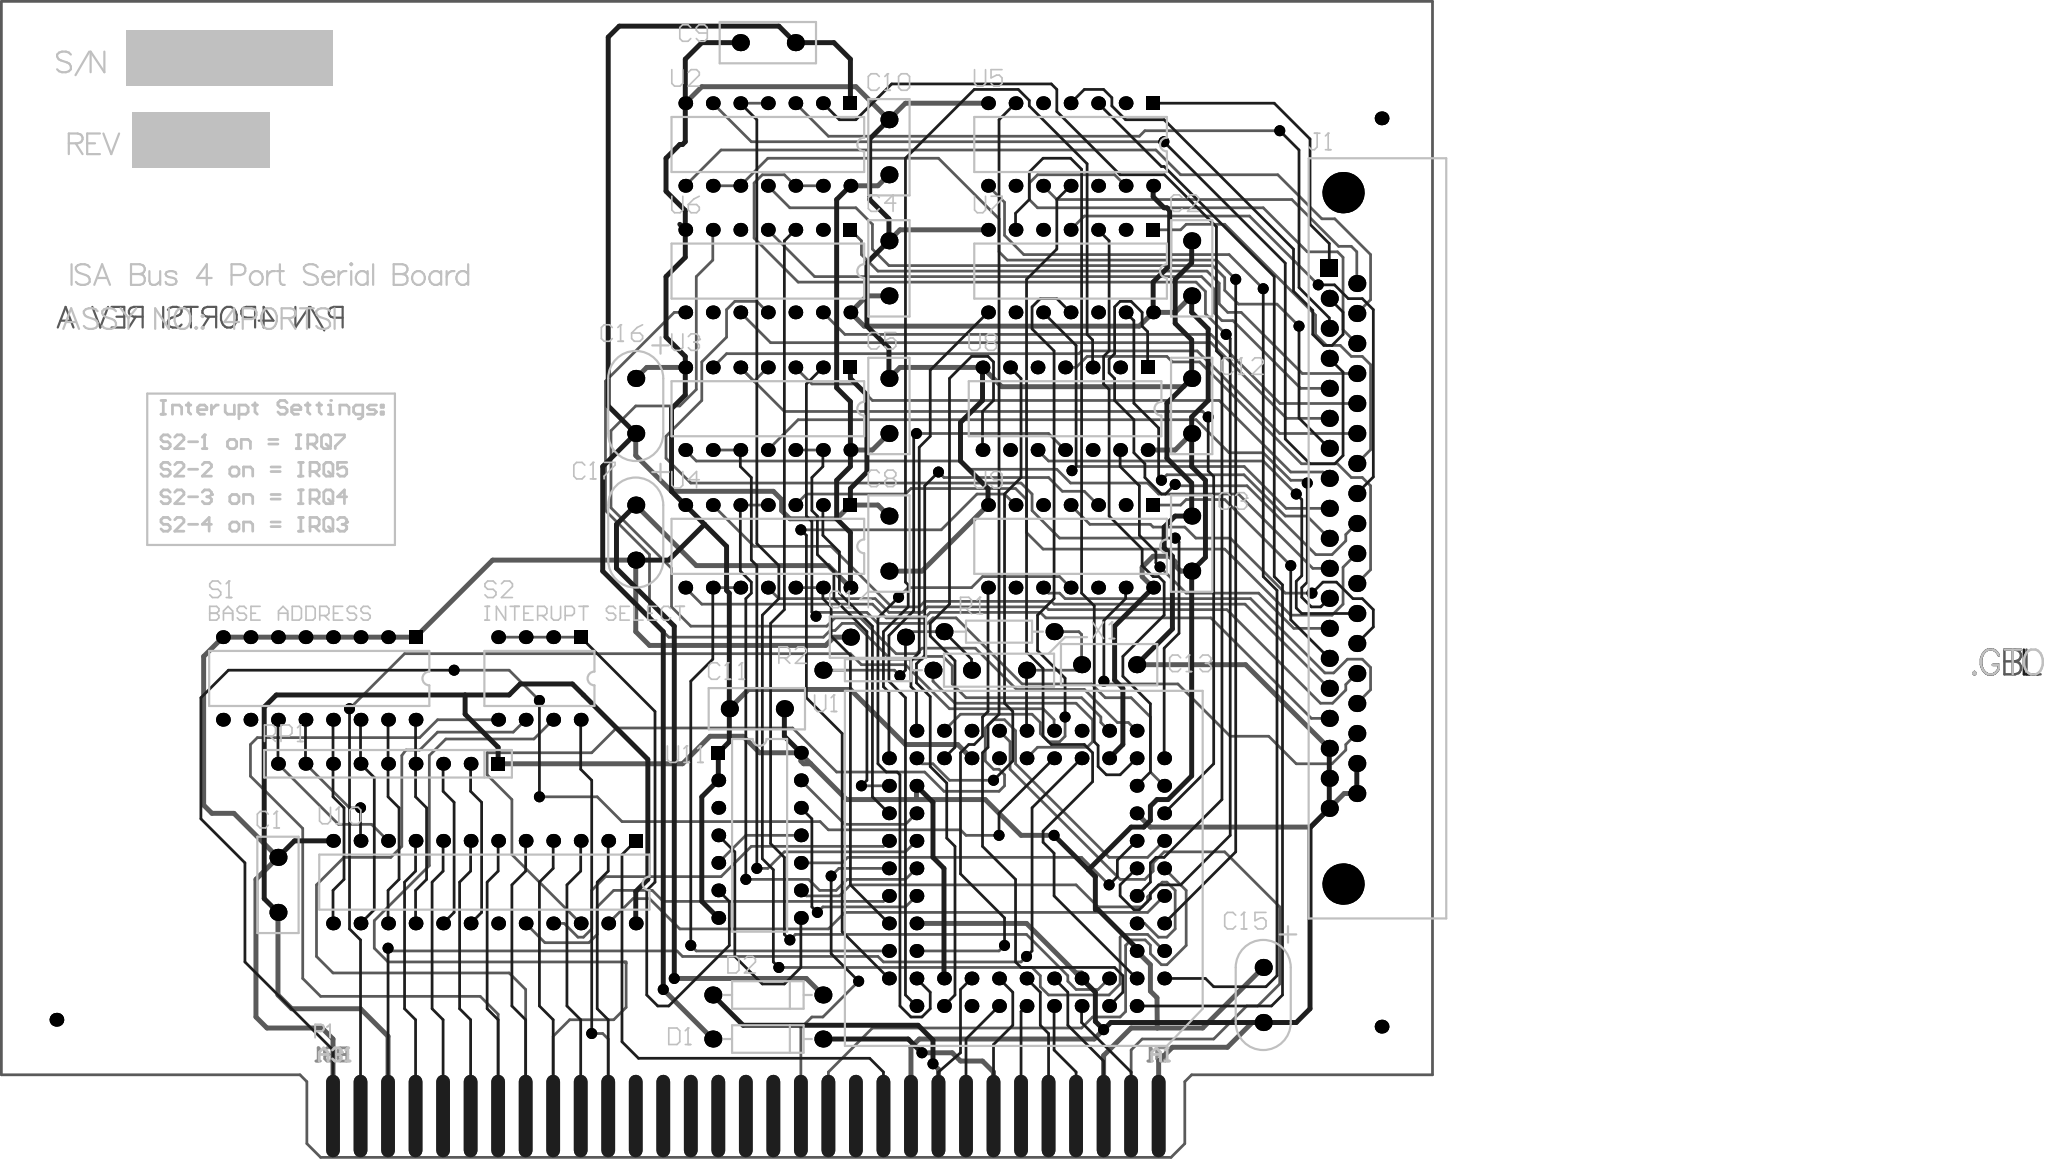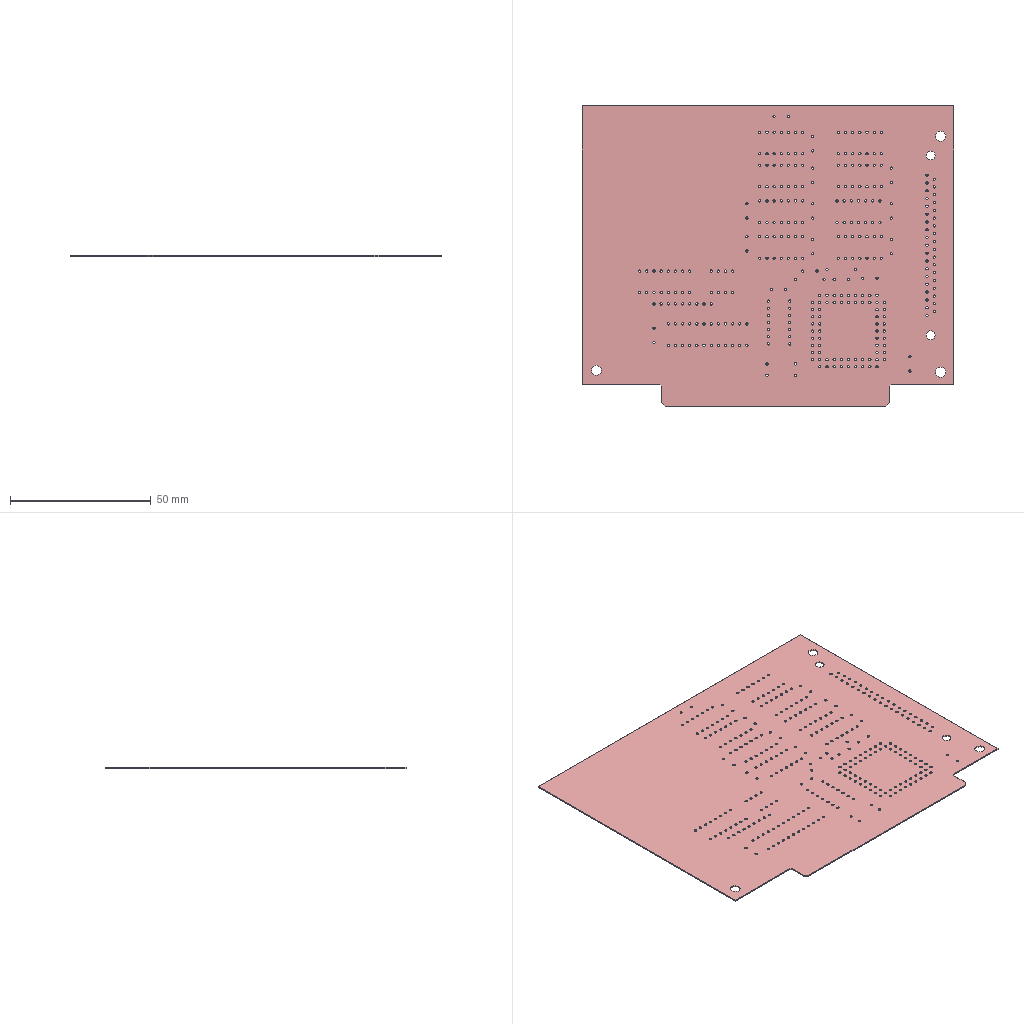Circuit board layout | Altium Designer | box 132.1 x 106.7 x 0.4 mm
Layer stack:
# Altium Designer layer stack of  (unit mm; dielectric type: 0 none, 1 core, 2 prepreg, 3 surface material)
index,name,kind,layer,copper_thickness_mm,dielectric_type,dielectric_thickness_mm,dielectric_material,dielectric_constant
0,TopPaste,other,,,,,,
1,TopOverlay,other,,,,,,
2,TopSolder,dielectric,,,3,0.0102,Solder Resist,3.5
3,TopLayer,copper,TopLayer,0.0356,,,,
4,Dielectric1,dielectric,,,1,0.32,FR-4,4.8
5,BottomLayer,copper,BottomLayer,0.0356,,,,
6,BottomSolder,dielectric,,,3,0.0102,Solder Resist,3.5
7,BottomOverlay,other,,,,,,
8,BottomPaste,other,,,,,,
# drill layer pairs: low layer,high layer
drill_pair,TopLayer,BottomLayer
Part placement:
Designator,Comment,Layer,Footprint,Center-X(mm),Center-Y(mm),Rotation
P1,CON AT62B,TopLayer,ECN-IBMXT,239.014,142.24,0
C9,0.1uF,TopLayer,RAD0.2,241.046,241.3,180
R2,1K5,TopLayer,AXIAL0.4,251.206,183.388,180
C13,20pF,TopLayer,RAD0.2,272.542,183.896,0
X1,1.843Mhz,TopLayer,XTAL1,262.382,183.388,360
J1,DB37,TopLayer,DB37RA/F,294.132,195.555,270
C17,10uF,TopLayer,TANT_2M/2M,228.854,196.088,270
U1,TL16C554,TopLayer,PGA68X11_SKT,264.922,165.1,270
U9,1489,TopLayer,DIP14,268.986,194.818,270
U3,1488,TopLayer,DIP14,241.046,207.518,270
U8,1489,TopLayer,DIP14,268.478,207.518,270
U7,1489,TopLayer,DIP14,268.986,220.218,270
U6,1489,TopLayer,DIP14,241.046,220.218,270
U2,1488,TopLayer,DIP14,241.046,231.902,270
U5,1489,TopLayer,DIP14,268.986,231.902,270
C10,0.1uF,TopLayer,RAD0.2,252.222,231.648,90
C2,0.1uF,TopLayer,RAD0.2,280.162,220.472,90
C3,0.1uF,TopLayer,RAD0.2,280.162,195.072,90
C12,0.1uF,TopLayer,RAD0.2,280.162,207.772,90
C4,0.1uF,TopLayer,RAD0.2,252.222,220.472,90
C5,0.1uF,TopLayer,RAD0.2,252.222,207.772,90
D2,1N4004,TopLayer,DIODE0.4,241.046,153.416,360
D1,1N4004,TopLayer,DIODE0.4,241.046,149.352,0
U10,P22V10,TopLayer,SDIP24,214.884,163.83,270
U11,74HC32,TopLayer,DIP14,240.284,168.148,360
C11,0.1uF,TopLayer,RAD0.2,240.03,179.832,180
S1,BASE ADDRESS,TopLayer,DIP16,199.644,182.626,270
S2,INTERUPT SELECT,TopLayer,DIP8,219.964,182.626,270
C8,0.1uF,TopLayer,RAD0.2,252.222,195.072,270
C1,0.1uF,TopLayer,RAD0.2,195.834,163.576,90
RP1,10K,TopLayer,SIP9,205.994,174.752,180
R1,1M,TopLayer,AXIAL0.4,262.382,186.944,360
C14,50pF,TopLayer,RAD0.2,251.206,186.436,180
U4,1488,TopLayer,DIP14,241.046,194.818,270
C16,10uF,TopLayer,TANT_2M/2M,228.854,207.772,270
C15,10uF,TopLayer,TANT_2M/2M,286.766,153.416,270
Pad and via stacks:
# Altium Designer via and pad stacks of  (unit mm). Each distinct definition once, with the count of objects using it.
# via: kind,start_layer,end_layer,hole_mm,diameter_mm,mode(0 simple;1 top-mid-bottom;2 full stack),diameter_per_layer,count,example_net
# pad: kind,layer,hole_mm,hole_type(0 round;1 square;2 slot),plating,top_size,top_shape(1 round;2 rect;3 octagon;9 rounded rect),mid_size,bottom_size,mode,footprint,size_per_layer,count,example
pad,TopLayer,0,0,plated,1.27x7.62,1,1.27x7.62,1.27x7.62,0,ECN-IBMXT,,31,P1.A31
pad,BottomLayer,0,0,plated,1.27x7.62,1,1.27x7.62,1.27x7.62,0,ECN-IBMXT,,31,P1.B31
pad,MultiLayer,0.8128,0,plated,1.575x1.575,1,1.575x1.575,1.575x1.575,0,RAD0.2,,24,C14.1
pad,MultiLayer,0.8128,0,plated,1.575x1.575,1,1.575x1.575,1.575x1.575,0,AXIAL0.4,,4,R2.1
pad,MultiLayer,0.8128,0,plated,1.575x1.575,1,1.575x1.575,1.575x1.575,0,XTAL1,,2,X1.2
pad,MultiLayer,3.175,0,plated,3.81x3.81,1,3.81x3.81,3.81x3.81,0,DB37RA/F,,2,J1.0
pad,MultiLayer,0.8128,0,plated,1.575x1.575,1,1.575x1.575,1.575x1.575,0,DB37RA/F,,36,J1.37
pad,MultiLayer,0.8128,0,plated,1.575x1.575,2,1.575x1.575,1.575x1.575,0,DB37RA/F,,1,J1.1
pad,MultiLayer,0.8128,0,plated,1.575x1.575,1,1.575x1.575,1.575x1.575,0,TANT 2M/2M,,6,C17.2
pad,MultiLayer,0.8128,0,plated,1.27x1.27,1,1.27x1.27,1.27x1.27,0,PGA68X11_SKT,,68,U1.2
pad,MultiLayer,0.8128,0,plated,1.27x1.27,1,1.27x1.27,1.27x1.27,0,DIP14,,117,U9.14
pad,MultiLayer,0.8128,0,plated,1.27x1.27,2,1.27x1.27,1.27x1.27,0,DIP14,,9,U9.1
pad,MultiLayer,0.8128,0,plated,1.575x1.575,1,1.575x1.575,1.575x1.575,0,DIODE0.4,,4,D2.A
pad,MultiLayer,0.8128,0,plated,1.27x1.27,2,1.27x1.27,1.27x1.27,0,SDIP24,,1,U10.1
pad,MultiLayer,0.8128,0,plated,1.27x1.27,1,1.27x1.27,1.27x1.27,0,SDIP24,,23,U10.2
pad,MultiLayer,0.8128,0,plated,1.27x1.27,1,1.27x1.27,1.27x1.27,0,SIP9,,8,RP1.9
pad,MultiLayer,0.8128,0,plated,1.27x1.27,2,1.27x1.27,1.27x1.27,0,SIP9,,1,RP1.1
pad,MultiLayer,3.556,0,plated,1.27x1.27,1,1.27x1.27,1.27x1.27,0,,,3,1
pad,MultiLayer,0.8128,0,plated,1.27x1.27,2,1.27x1.27,1.27x1.27,0,DIP16,,1,S1.1
pad,MultiLayer,0.8128,0,plated,1.27x1.27,1,1.27x1.27,1.27x1.27,0,DIP16,,15,S1.2
pad,MultiLayer,0.8128,0,plated,1.27x1.27,2,1.27x1.27,1.27x1.27,0,DIP8,,1,S2.1
pad,MultiLayer,0.8128,0,plated,1.27x1.27,1,1.27x1.27,1.27x1.27,0,DIP8,,7,S2.2
via,TopLayer,BottomLayer,0.5588,1.016,0,,52,A2
Design rules, without the lines most boards share:
# Altium Designer design rules of  (exported by Altium Designer, unit mm)
# columns: name | kind | enabled | priority | scope1 | scope2 | descriptor | typed fields (field=value)
HoleToHoleClearance | 52 | enabled | 1 | All | All | Hole To Hole Clearance (Gap=10mil) (All),(All) | gap=0.254
DiffPairsRouting | 51 | enabled | 1 | All | All | Differential Pairs Uncoupled Length using the Gap Constraints (Min=10mil) (Max=10mil) (Prefered=10mil)  and Width Constraints (Min=15mil) (Max=15mil) (Prefered=15mil) (All) |
All | 2 | enabled | 7 | All | All | Width Constraint (Min=10mil) (Max=10mil) (Preferred=10mil) (All) |
Testpoint | 43 | disabled | 1 | All | All | Fabrication Testpoint Style (Under Component=Yes) (Disabled)(All) |
TestPointUsage | 44 | disabled | 1 | All | All | Fabrication Testpoint Usage (Valid =One Required, Allow multiple per net=No) (Disabled)(All) |
SolderMaskExpansion_Mtg | 13 | enabled | 1 | InPadClass('MTG') | All | Solder Mask Expansion (Expansion =50mil) (InPadClass('MTG')) | expansion=1.27
SupplyNets | 41 | enabled | 2 | InNet('GND') | All | Supply Net(s)(InNet('GND')) |
SupplyNets_1 | 41 | enabled | 1 | InNet('VCC') | All | Supply Net(s)(InNet('VCC')) |
PolygonConnect | 20 | enabled | 1 | All | All | Polygon Connect Rule(Relief Connect )(Conductor Width=10mil) (Relief Angle=90 Angle) (Entries=4) (Air Gap Width=10mil) (All),(All) | connect_style(0=relief,1=direct,2=none)=0 relief_conductor_width=0.254 relief_entries=4
PlaneConnect | 6 | enabled | 1 | All | All | Power Plane Connect Rule(Relief Connect )(Expansion=20mil) (Conductor Width=10mil) (Air Gap=10mil) (Entries=4) (All) | relief_conductor_width=0.254 relief_entries=4 relief_expansion=0.508
Clearance | 0 | enabled | 1 | All | All | Clearance Constraint (Gap=10mil) (All),(All) | gap=0.254
SolderMaskExpansion | 13 | enabled | 2 | All | All | Solder Mask Expansion (Expansion =4mil) (All) | expansion=0.1016
PasteMaskExpansion | 14 | enabled | 2 | All | All | Paste Mask Expansion (Expansion =0mil) (All) | expansion=0
RoutingVias | 11 | enabled | 1 | All | All | Routing Via (MinHoleWidth=22mil) (MaxHoleWidth=28mil) (PreferredHoleWidth=22mil) (MinWidth=40mil) (MaxWidth=50mil) (PreferedWidth=40mil) (All) | via_min_hole=0.5588 via_max_hole=0.7112 via_preferred_diameter=1.016 via_preferred_hole=0.5588
PasteMaskExpansion_Edge | 14 | enabled | 1 | InComponent('P1') | All | Paste Mask Expansion (Expansion =-150mil) (InComponent('P1')) | expansion=-3.81
MinimumAnnularRing | 19 | enabled | 2 | All | All | Minimum Annular Ring (Minimum=9mil) (All) |
MinimumAnnularRing_Mtg | 19 | enabled | 1 | InPadClass('MTG') | All | Minimum Annular Ring (Minimum=-90mil) (InPadClass('MTG')) |
ComponentClearance | 24 | disabled | 1 | All | All | Component Clearance Constraint ( Horizontal Gap = 10mil, Vertical Gap = 10mil ) (Disabled)(All),(All)  | gap=0.254
HoleSize | 42 | enabled | 1 | All | All | Hole Size Constraint (Min=1mil) (Max=140mil) (All) |
+12V_U/P | 2 | enabled | 6 | InNet('+12V_U/P') | All | Width Constraint (Min=18mil) (Max=18mil) (Preferred=18mil) (InNet('+12V_U/P')) |
-12V_U/P | 2 | enabled | 5 | InNet('-12V_U/P') | All | Width Constraint (Min=18mil) (Max=18mil) (Preferred=18mil) (InNet('-12V_U/P')) |
-12V | 2 | enabled | 4 | InNet('-12V') | All | Width Constraint (Min=18mil) (Max=18mil) (Preferred=18mil) (InNet('-12V')) |
GND | 2 | enabled | 3 | InNet('GND') | All | Width Constraint (Min=18mil) (Max=18mil) (Preferred=18mil) (InNet('GND')) |
VCC | 2 | enabled | 2 | InNet('VCC') | All | Width Constraint (Min=18mil) (Max=18mil) (Preferred=18mil) (InNet('VCC')) |
+12V | 2 | enabled | 1 | InNet('+12V') | All | Width Constraint (Min=18mil) (Max=18mil) (Preferred=18mil) (InNet('+12V')) |
Classes set for this board:
# Altium Designer classes of  (member kind: 0 net, 1 component, 2 from-to, 3 pad, 4 layer, 5 differential pair, 6 design channel, 7 polygon, 8 structure, 9 xSignal)
# columns: class name | member kind | superclass | members
MTG | 3 | no | Free-3; Free-2; Free-1;
A[0..2] | 0 | no | A0; A1; A2;
D[0..7] | 0 | no | D0; D1; D2; D3; D4; D5; D6; D7;